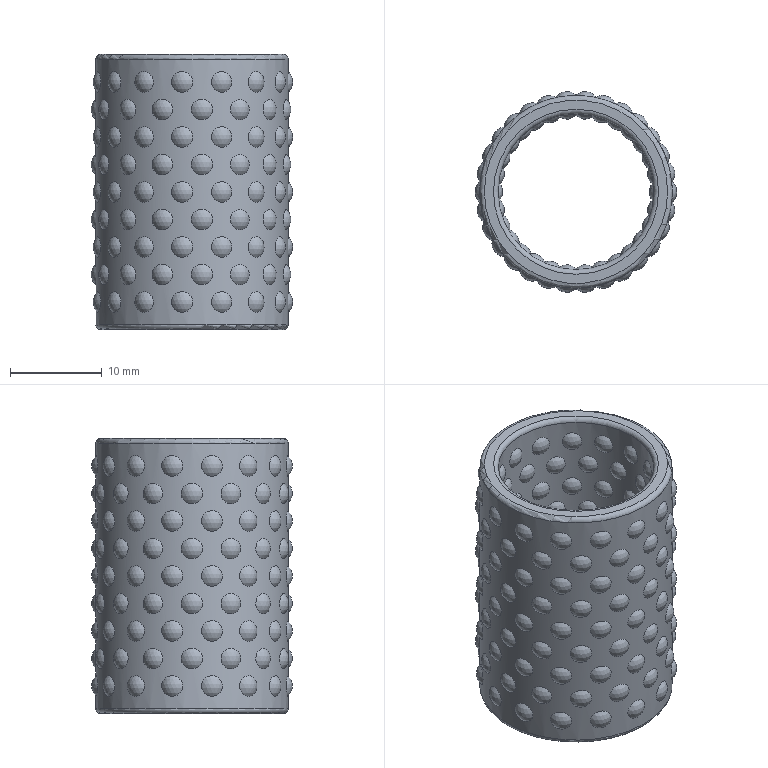Part | STEP file | 200 mesh_id1794 | 1 solid | 278 faces | box 22 x 21.896 x 30 mm | volume 3861 mm3 | sphere 270 | torus 4 | cylinder 2 | plane 2 | commonest cylinder face diameters 17 x1 21 x1